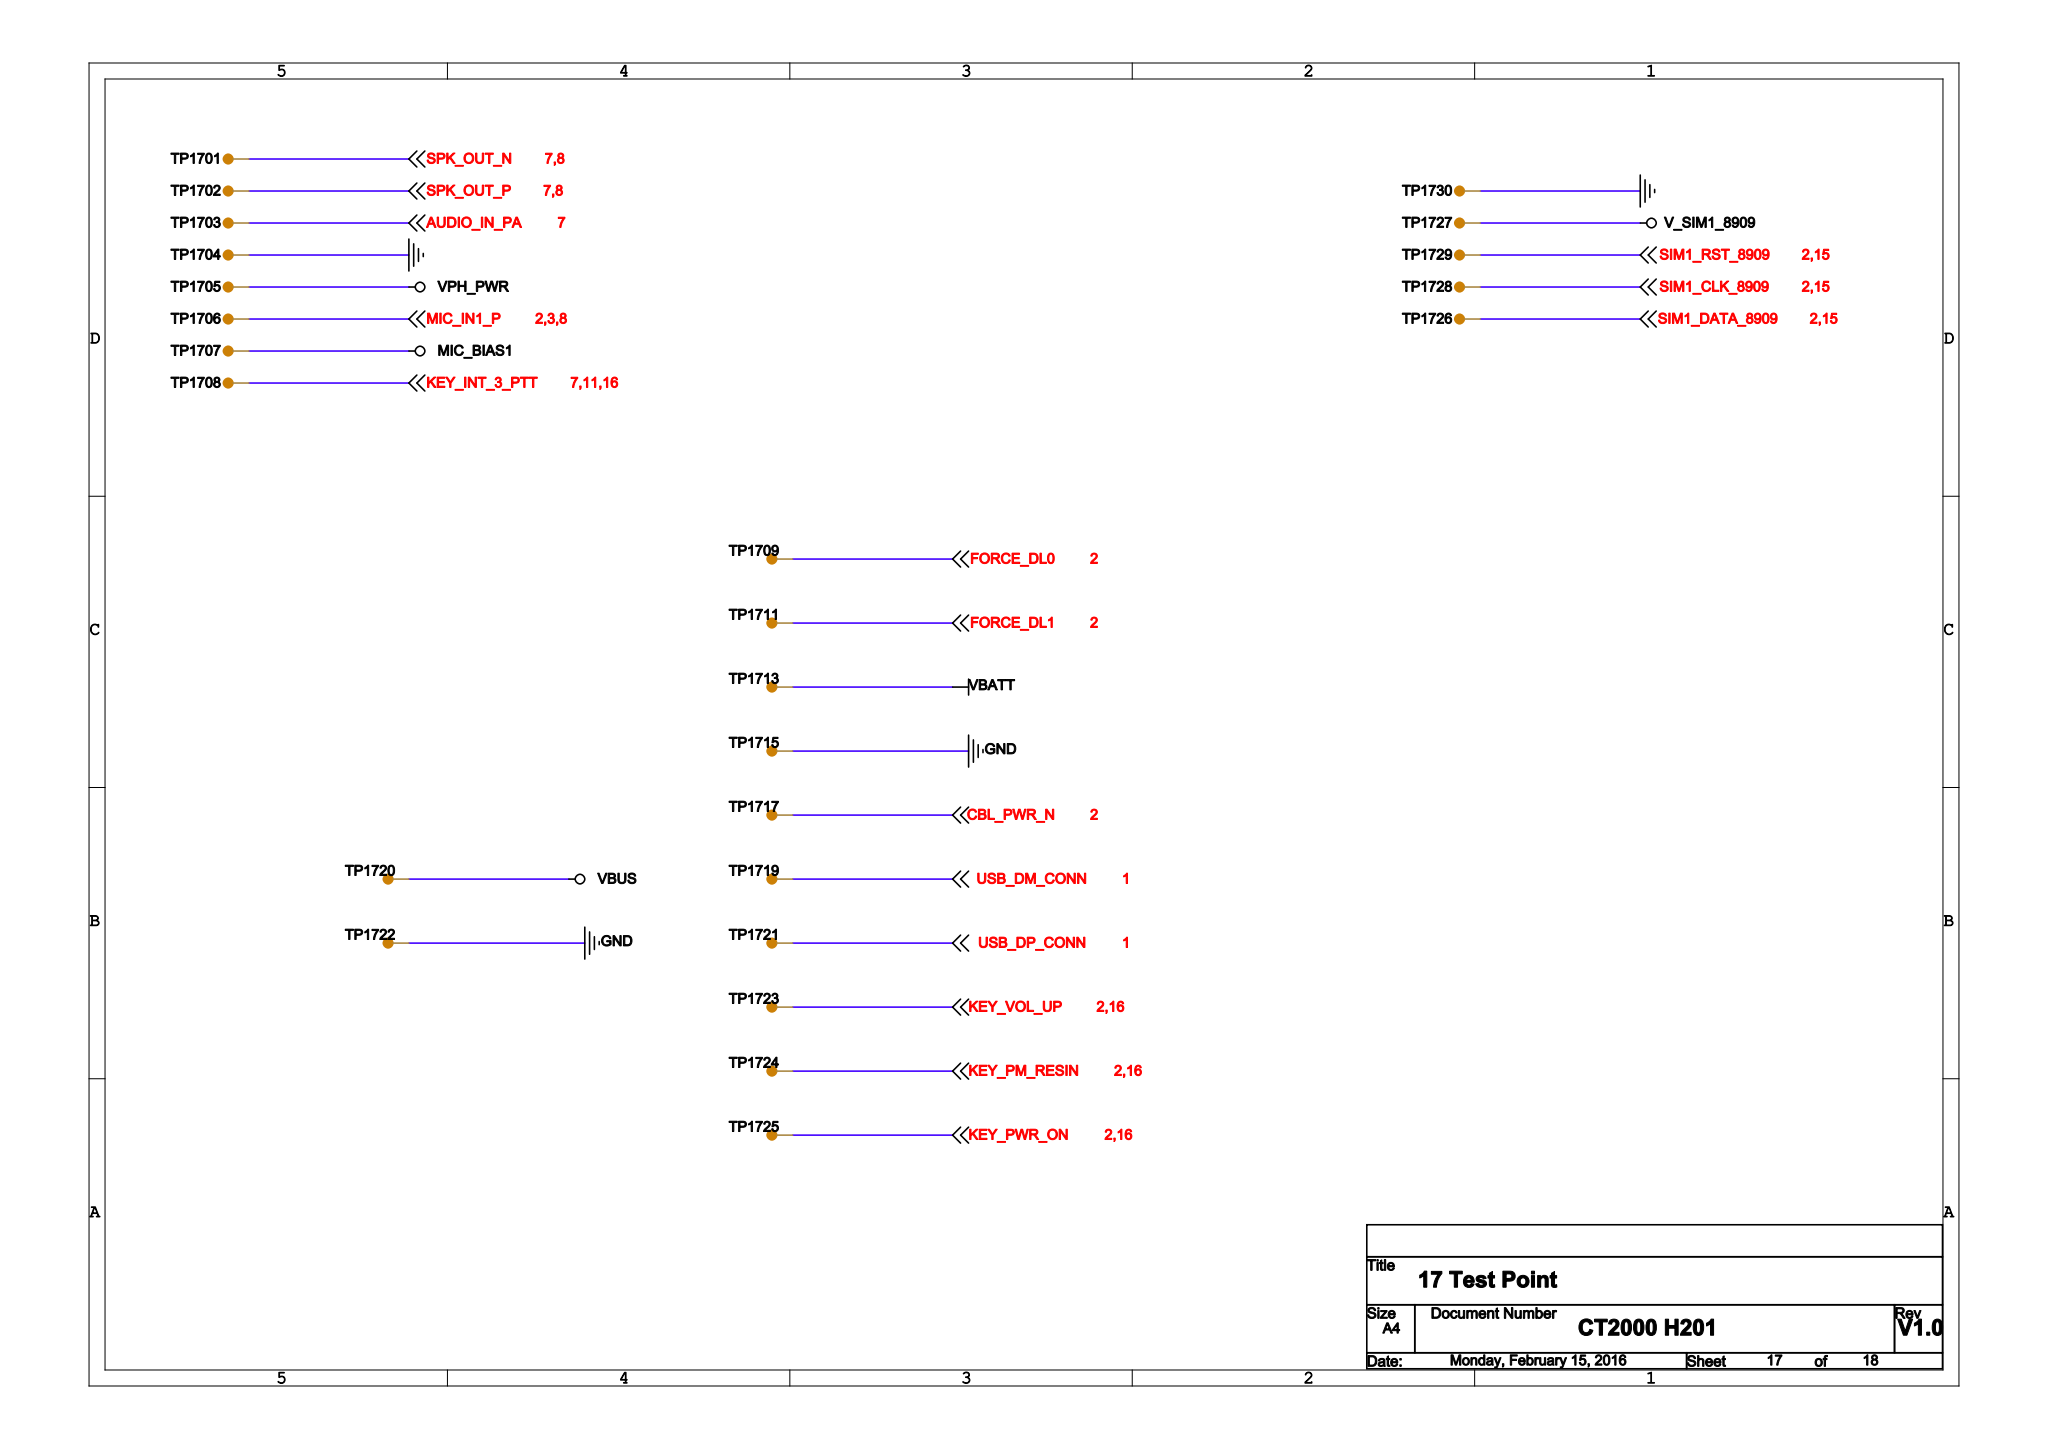Circuit board | Cadence Allegro | 573 parts | 376 nets | one sheet of the schematic
Parts on this sheet (reference | value | footprint):
TP1701 | 1 mm | TESTPOINT_32MIL
TP1702 | 1 mm | TESTPOINT_32MIL
TP1703 | 1 mm | TESTPOINT_32MIL
TP1704 | 1 mm | TESTPOINT_32MIL
TP1705 | 1 mm | TESTPOINT_32MIL
TP1706 | 1 mm | TESTPOINT_32MIL
TP1707 | 1 mm | TESTPOINT_32MIL
TP1708 | 1 mm | TESTPOINT_32MIL
TP1709 | 1 mm | TESTPOINT_32MIL
TP1711 | 1 mm | TESTPOINT_32MIL
TP1713 | 1 mm | TESTPOINT_32MIL
TP1715 | 1 mm | TESTPOINT_32MIL
TP1717 | 1 mm | TESTPOINT_32MIL
TP1719 | 1 mm | TESTPOINT_32MIL
TP1720 | 1 mm | TESTPOINT_32MIL
TP1721 | 1 mm | TESTPOINT_32MIL
TP1722 | 1 mm | TESTPOINT_32MIL
TP1723 | 1 mm | TESTPOINT_32MIL
TP1724 | 1 mm | TESTPOINT_32MIL
TP1725 | 1 mm | TESTPOINT_32MIL
TP1726 | 1 mm | TESTPOINT_32MIL
TP1727 | 1 mm | TESTPOINT_32MIL
TP1728 | 1 mm | TESTPOINT_32MIL
TP1729 | 1 mm | TESTPOINT_32MIL
TP1730 | 1 mm | TESTPOINT_32MIL
Nets of these parts (net: part-pin ...):
GND: TP1704-1 TP1715-1 TP1722-1 TP1730-1
MIC_IN1_P: TP1706-1
KEY_INT_3_PTT: TP1708-1
KEY_PM_RESIN: TP1724-1
KEY_VOL_UP: TP1723-1
VBATT: TP1713-1
MIC_BIAS1: TP1707-1
VPH_PWR: TP1705-1
KEY_PWR_ON: TP1725-1
V_SIM1_8909: TP1727-1
USB_DP_CONN: TP1721-1
USB_DM_CONN: TP1719-1
VBUS: TP1720-1
CBL_PWR_N: TP1717-1
FORCE_DL0: TP1709-1
FORCE_DL1: TP1711-1
SIM1_CLK_8909: TP1728-1
SIM1_DATA_8909: TP1726-1
SIM1_RST_8909: TP1729-1
SPK_OUT_N: TP1701-1
SPK_OUT_P: TP1702-1
AUDIO_IN_PA: TP1703-1